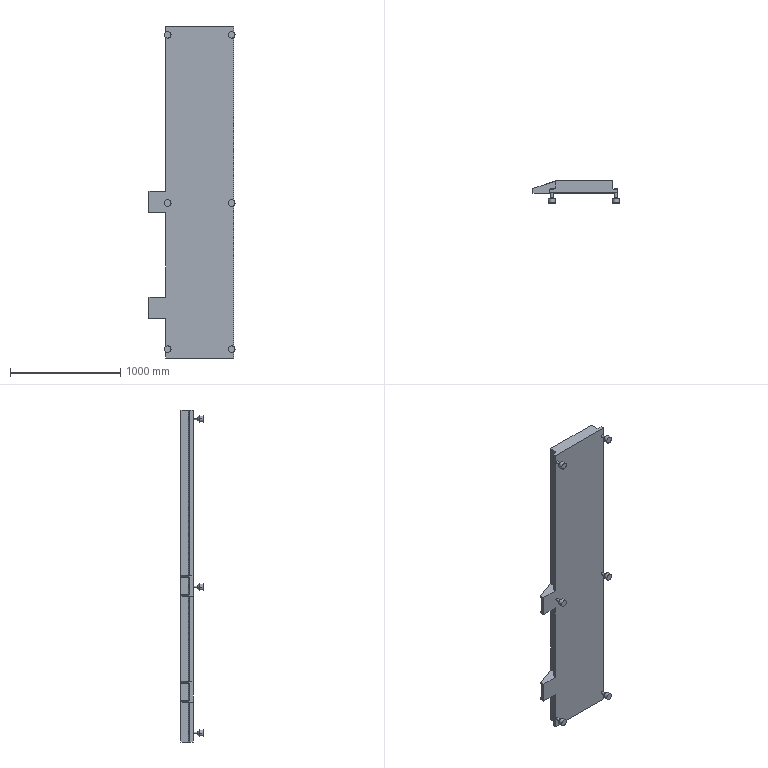Part | Creo | features PROTRUSION 8, CURVE 6, CHAMFER 3, DATUM PLANE 3, MOVE 2, COORDINATE SYSTEM 1, CUT 1 | 1 solid | 111 faces | box 780 x 200 x 3010 mm | volume 141202284 mm3 | plane 63 | cylinder 36 | cone 12 | commonest cylinder face diameters 24 x24 60 x12